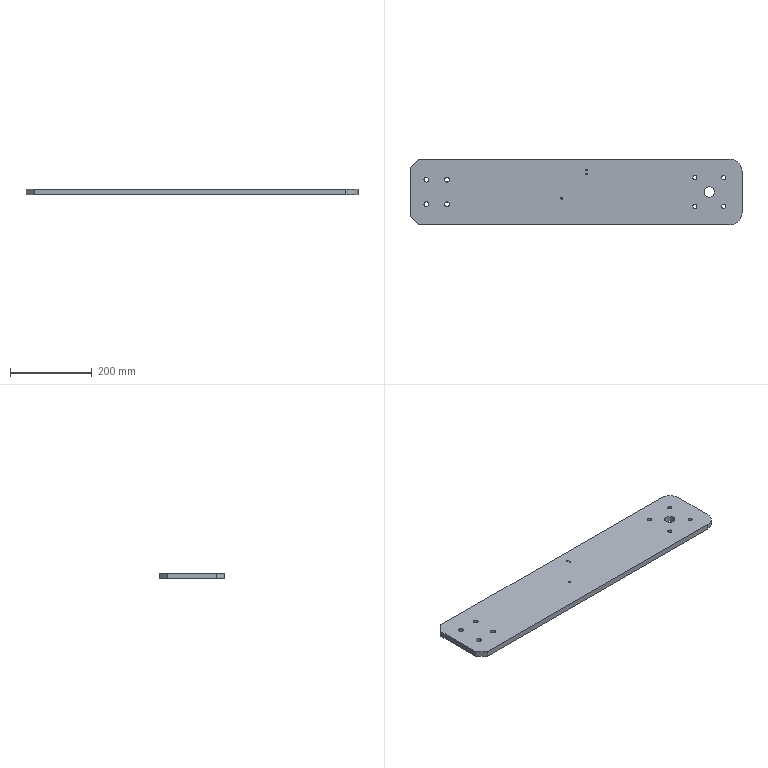Part | STEP file | Head plate 2 | 1 solid | 34 faces | box 810 x 160 x 14 mm | volume 1785161 mm3 | cylinder 26 | plane 8 | commonest cylinder face diameters 10 x8 12 x8 4 x4 5 x2 25 x2 60 x2
STEP:
#1=CARTESIAN_POINT('',(312.5,0.,14.));
#2=VERTEX_POINT('',#1);
#3=CARTESIAN_POINT('',(337.5,0.,14.));
#4=VERTEX_POINT('',#3);
#5=CARTESIAN_POINT('',(325.,0.,14.));
#6=DIRECTION('',(0.,0.,1.));
#7=DIRECTION('',(-1.,0.,0.));
#8=AXIS2_PLACEMENT_3D('',#5,#6,#7);
#9=CIRCLE('',#8,12.5);
#10=EDGE_CURVE('',#2,#4,#9,.T.);
#11=ORIENTED_EDGE('',*,*,#10,.T.);
#12=CARTESIAN_POINT('',(337.5,0.,0.));
#13=VERTEX_POINT('',#12);
#14=CARTESIAN_POINT('',(337.5,0.,14.));
#15=DIRECTION('',(0.,0.,-1.));
#16=VECTOR('',#15,1000.);
#17=LINE('',#14,#16);
#18=EDGE_CURVE('',#4,#13,#17,.T.);
#19=ORIENTED_EDGE('',*,*,#18,.T.);
#20=CARTESIAN_POINT('',(312.5,0.,0.));
#21=VERTEX_POINT('',#20);
#22=CARTESIAN_POINT('',(325.,0.,0.));
#23=DIRECTION('',(0.,0.,1.));
#24=DIRECTION('',(-1.,0.,0.));
#25=AXIS2_PLACEMENT_3D('',#22,#23,#24);
#26=CIRCLE('',#25,12.5);
#27=EDGE_CURVE('',#21,#13,#26,.T.);
#28=ORIENTED_EDGE('',*,*,#27,.F.);
#29=CARTESIAN_POINT('',(312.5,0.,14.));
#30=DIRECTION('',(0.,0.,-1.));
#31=VECTOR('',#30,1000.);
#32=LINE('',#29,#31);
#33=EDGE_CURVE('',#2,#21,#32,.T.);
#34=ORIENTED_EDGE('',*,*,#33,.F.);
#35=EDGE_LOOP('',(#11,#19,#28,#34));
#36=FACE_OUTER_BOUND('',#35,.T.);
#37=CARTESIAN_POINT('',(325.,0.,14.));
#38=DIRECTION('',(0.,0.,-1.));
#39=DIRECTION('',(-1.,0.,0.));
#40=AXIS2_PLACEMENT_3D('',#37,#38,#39);
#41=CYLINDRICAL_SURFACE('',#40,12.5);
#42=ADVANCED_FACE('',(#36),#41,.F.);
#43=CARTESIAN_POINT('',(355.,35.,14.));
#44=VERTEX_POINT('',#43);
#45=CARTESIAN_POINT('',(365.,35.,14.));
#46=VERTEX_POINT('',#45);
#47=CARTESIAN_POINT('',(360.,35.,14.));
#48=DIRECTION('',(0.,0.,1.));
#49=DIRECTION('',(-1.,0.,0.));
#50=AXIS2_PLACEMENT_3D('',#47,#48,#49);
#51=CIRCLE('',#50,5.);
#52=EDGE_CURVE('',#44,#46,#51,.T.);
#53=ORIENTED_EDGE('',*,*,#52,.T.);
#54=CARTESIAN_POINT('',(365.,35.,0.));
#55=VERTEX_POINT('',#54);
#56=CARTESIAN_POINT('',(365.,35.,14.));
#57=DIRECTION('',(0.,0.,-1.));
#58=VECTOR('',#57,1000.);
#59=LINE('',#56,#58);
#60=EDGE_CURVE('',#46,#55,#59,.T.);
#61=ORIENTED_EDGE('',*,*,#60,.T.);
#62=CARTESIAN_POINT('',(355.,35.,0.));
#63=VERTEX_POINT('',#62);
#64=CARTESIAN_POINT('',(360.,35.,0.));
#65=DIRECTION('',(0.,0.,1.));
#66=DIRECTION('',(-1.,0.,0.));
#67=AXIS2_PLACEMENT_3D('',#64,#65,#66);
#68=CIRCLE('',#67,5.);
#69=EDGE_CURVE('',#63,#55,#68,.T.);
#70=ORIENTED_EDGE('',*,*,#69,.F.);
#71=CARTESIAN_POINT('',(355.,35.,14.));
#72=DIRECTION('',(0.,0.,-1.));
#73=VECTOR('',#72,1000.);
#74=LINE('',#71,#73);
#75=EDGE_CURVE('',#44,#63,#74,.T.);
#76=ORIENTED_EDGE('',*,*,#75,.F.);
#77=EDGE_LOOP('',(#53,#61,#70,#76));
#78=FACE_OUTER_BOUND('',#77,.T.);
#79=CARTESIAN_POINT('',(360.,35.,14.));
#80=DIRECTION('',(0.,0.,-1.));
#81=DIRECTION('',(-1.,0.,0.));
#82=AXIS2_PLACEMENT_3D('',#79,#80,#81);
#83=CYLINDRICAL_SURFACE('',#82,5.);
#84=ADVANCED_FACE('',(#78),#83,.F.);
#85=CARTESIAN_POINT('',(285.,35.,14.));
#86=VERTEX_POINT('',#85);
#87=CARTESIAN_POINT('',(295.,35.,14.));
#88=VERTEX_POINT('',#87);
#89=CARTESIAN_POINT('',(290.,35.,14.));
#90=DIRECTION('',(0.,0.,1.));
#91=DIRECTION('',(-1.,0.,0.));
#92=AXIS2_PLACEMENT_3D('',#89,#90,#91);
#93=CIRCLE('',#92,5.);
#94=EDGE_CURVE('',#86,#88,#93,.T.);
#95=ORIENTED_EDGE('',*,*,#94,.T.);
#96=CARTESIAN_POINT('',(295.,35.,0.));
#97=VERTEX_POINT('',#96);
#98=CARTESIAN_POINT('',(295.,35.,14.));
#99=DIRECTION('',(0.,0.,-1.));
#100=VECTOR('',#99,1000.);
#101=LINE('',#98,#100);
#102=EDGE_CURVE('',#88,#97,#101,.T.);
#103=ORIENTED_EDGE('',*,*,#102,.T.);
#104=CARTESIAN_POINT('',(285.,35.,0.));
#105=VERTEX_POINT('',#104);
#106=CARTESIAN_POINT('',(290.,35.,0.));
#107=DIRECTION('',(0.,0.,1.));
#108=DIRECTION('',(-1.,0.,0.));
#109=AXIS2_PLACEMENT_3D('',#106,#107,#108);
#110=CIRCLE('',#109,5.);
#111=EDGE_CURVE('',#105,#97,#110,.T.);
#112=ORIENTED_EDGE('',*,*,#111,.F.);
#113=CARTESIAN_POINT('',(285.,35.,14.));
#114=DIRECTION('',(0.,0.,-1.));
#115=VECTOR('',#114,1000.);
#116=LINE('',#113,#115);
#117=EDGE_CURVE('',#86,#105,#116,.T.);
#118=ORIENTED_EDGE('',*,*,#117,.F.);
#119=EDGE_LOOP('',(#95,#103,#112,#118));
#120=FACE_OUTER_BOUND('',#119,.T.);
#121=CARTESIAN_POINT('',(290.,35.,14.));
#122=DIRECTION('',(0.,0.,-1.));
#123=DIRECTION('',(-1.,0.,0.));
#124=AXIS2_PLACEMENT_3D('',#121,#122,#123);
#125=CYLINDRICAL_SURFACE('',#124,5.);
#126=ADVANCED_FACE('',(#120),#125,.F.);
#127=CARTESIAN_POINT('',(285.,-35.,14.));
#128=VERTEX_POINT('',#127);
#129=CARTESIAN_POINT('',(295.,-35.,14.));
#130=VERTEX_POINT('',#129);
#131=CARTESIAN_POINT('',(290.,-35.,14.));
#132=DIRECTION('',(0.,0.,1.));
#133=DIRECTION('',(-1.,0.,0.));
#134=AXIS2_PLACEMENT_3D('',#131,#132,#133);
#135=CIRCLE('',#134,5.);
#136=EDGE_CURVE('',#128,#130,#135,.T.);
#137=ORIENTED_EDGE('',*,*,#136,.T.);
#138=CARTESIAN_POINT('',(295.,-35.,0.));
#139=VERTEX_POINT('',#138);
#140=CARTESIAN_POINT('',(295.,-35.,14.));
#141=DIRECTION('',(0.,0.,-1.));
#142=VECTOR('',#141,1000.);
#143=LINE('',#140,#142);
#144=EDGE_CURVE('',#130,#139,#143,.T.);
#145=ORIENTED_EDGE('',*,*,#144,.T.);
#146=CARTESIAN_POINT('',(285.,-35.,0.));
#147=VERTEX_POINT('',#146);
#148=CARTESIAN_POINT('',(290.,-35.,0.));
#149=DIRECTION('',(0.,0.,1.));
#150=DIRECTION('',(-1.,0.,0.));
#151=AXIS2_PLACEMENT_3D('',#148,#149,#150);
#152=CIRCLE('',#151,5.);
#153=EDGE_CURVE('',#147,#139,#152,.T.);
#154=ORIENTED_EDGE('',*,*,#153,.F.);
#155=CARTESIAN_POINT('',(285.,-35.,14.));
#156=DIRECTION('',(0.,0.,-1.));
#157=VECTOR('',#156,1000.);
#158=LINE('',#155,#157);
#159=EDGE_CURVE('',#128,#147,#158,.T.);
#160=ORIENTED_EDGE('',*,*,#159,.F.);
#161=EDGE_LOOP('',(#137,#145,#154,#160));
#162=FACE_OUTER_BOUND('',#161,.T.);
#163=CARTESIAN_POINT('',(290.,-35.,14.));
#164=DIRECTION('',(0.,0.,-1.));
#165=DIRECTION('',(-1.,0.,0.));
#166=AXIS2_PLACEMENT_3D('',#163,#164,#165);
#167=CYLINDRICAL_SURFACE('',#166,5.);
#168=ADVANCED_FACE('',(#162),#167,.F.);
#169=CARTESIAN_POINT('',(355.,-35.,14.));
#170=VERTEX_POINT('',#169);
#171=CARTESIAN_POINT('',(365.,-35.,14.));
#172=VERTEX_POINT('',#171);
#173=CARTESIAN_POINT('',(360.,-35.,14.));
#174=DIRECTION('',(0.,0.,1.));
#175=DIRECTION('',(-1.,0.,0.));
#176=AXIS2_PLACEMENT_3D('',#173,#174,#175);
#177=CIRCLE('',#176,5.);
#178=EDGE_CURVE('',#170,#172,#177,.T.);
#179=ORIENTED_EDGE('',*,*,#178,.T.);
#180=CARTESIAN_POINT('',(365.,-35.,0.));
#181=VERTEX_POINT('',#180);
#182=CARTESIAN_POINT('',(365.,-35.,14.));
#183=DIRECTION('',(0.,0.,-1.));
#184=VECTOR('',#183,1000.);
#185=LINE('',#182,#184);
#186=EDGE_CURVE('',#172,#181,#185,.T.);
#187=ORIENTED_EDGE('',*,*,#186,.T.);
#188=CARTESIAN_POINT('',(355.,-35.,0.));
#189=VERTEX_POINT('',#188);
#190=CARTESIAN_POINT('',(360.,-35.,0.));
#191=DIRECTION('',(0.,0.,1.));
#192=DIRECTION('',(-1.,0.,0.));
#193=AXIS2_PLACEMENT_3D('',#190,#191,#192);
#194=CIRCLE('',#193,5.);
#195=EDGE_CURVE('',#189,#181,#194,.T.);
#196=ORIENTED_EDGE('',*,*,#195,.F.);
#197=CARTESIAN_POINT('',(355.,-35.,14.));
#198=DIRECTION('',(0.,0.,-1.));
#199=VECTOR('',#198,1000.);
#200=LINE('',#197,#199);
#201=EDGE_CURVE('',#170,#189,#200,.T.);
#202=ORIENTED_EDGE('',*,*,#201,.F.);
#203=EDGE_LOOP('',(#179,#187,#196,#202));
#204=FACE_OUTER_BOUND('',#203,.T.);
#205=CARTESIAN_POINT('',(360.,-35.,14.));
#206=DIRECTION('',(0.,0.,-1.));
#207=DIRECTION('',(-1.,0.,0.));
#208=AXIS2_PLACEMENT_3D('',#205,#206,#207);
#209=CYLINDRICAL_SURFACE('',#208,5.);
#210=ADVANCED_FACE('',(#204),#209,.F.);
#211=CARTESIAN_POINT('',(-37.5,-15.,0.));
#212=VERTEX_POINT('',#211);
#213=CARTESIAN_POINT('',(-32.5,-15.,0.));
#214=VERTEX_POINT('',#213);
#215=CARTESIAN_POINT('',(-35.,-15.,0.));
#216=DIRECTION('',(0.,0.,1.));
#217=DIRECTION('',(1.,0.,0.));
#218=AXIS2_PLACEMENT_3D('',#215,#216,#217);
#219=CIRCLE('',#218,2.5);
#220=EDGE_CURVE('',#212,#214,#219,.T.);
#221=ORIENTED_EDGE('',*,*,#220,.F.);
#222=CARTESIAN_POINT('',(-37.5,-15.,14.));
#223=VERTEX_POINT('',#222);
#224=CARTESIAN_POINT('',(-37.5,-15.,-1.));
#225=DIRECTION('',(0.,0.,1.));
#226=VECTOR('',#225,1000.);
#227=LINE('',#224,#226);
#228=EDGE_CURVE('',#212,#223,#227,.T.);
#229=ORIENTED_EDGE('',*,*,#228,.T.);
#230=CARTESIAN_POINT('',(-32.5,-15.,14.));
#231=VERTEX_POINT('',#230);
#232=CARTESIAN_POINT('',(-35.,-15.,14.));
#233=DIRECTION('',(0.,0.,1.));
#234=DIRECTION('',(1.,0.,0.));
#235=AXIS2_PLACEMENT_3D('',#232,#233,#234);
#236=CIRCLE('',#235,2.5);
#237=EDGE_CURVE('',#223,#231,#236,.T.);
#238=ORIENTED_EDGE('',*,*,#237,.T.);
#239=CARTESIAN_POINT('',(-32.5,-15.,-1.));
#240=DIRECTION('',(0.,0.,1.));
#241=VECTOR('',#240,1000.);
#242=LINE('',#239,#241);
#243=EDGE_CURVE('',#214,#231,#242,.T.);
#244=ORIENTED_EDGE('',*,*,#243,.F.);
#245=EDGE_LOOP('',(#221,#229,#238,#244));
#246=FACE_OUTER_BOUND('',#245,.T.);
#247=CARTESIAN_POINT('',(-35.,-15.,-1.));
#248=DIRECTION('',(0.,0.,1.));
#249=DIRECTION('',(1.,0.,0.));
#250=AXIS2_PLACEMENT_3D('',#247,#248,#249);
#251=CYLINDRICAL_SURFACE('',#250,2.5);
#252=ADVANCED_FACE('',(#246),#251,.F.);
#253=CARTESIAN_POINT('',(-371.,30.,0.));
#254=VERTEX_POINT('',#253);
#255=CARTESIAN_POINT('',(-359.,30.,0.));
#256=VERTEX_POINT('',#255);
#257=CARTESIAN_POINT('',(-365.,30.,0.));
#258=DIRECTION('',(0.,0.,1.));
#259=DIRECTION('',(1.,0.,0.));
#260=AXIS2_PLACEMENT_3D('',#257,#258,#259);
#261=CIRCLE('',#260,6.);
#262=EDGE_CURVE('',#254,#256,#261,.T.);
#263=ORIENTED_EDGE('',*,*,#262,.F.);
#264=CARTESIAN_POINT('',(-371.,30.,14.));
#265=VERTEX_POINT('',#264);
#266=CARTESIAN_POINT('',(-371.,30.,-1.));
#267=DIRECTION('',(0.,0.,1.));
#268=VECTOR('',#267,1000.);
#269=LINE('',#266,#268);
#270=EDGE_CURVE('',#254,#265,#269,.T.);
#271=ORIENTED_EDGE('',*,*,#270,.T.);
#272=CARTESIAN_POINT('',(-359.,30.,14.));
#273=VERTEX_POINT('',#272);
#274=CARTESIAN_POINT('',(-365.,30.,14.));
#275=DIRECTION('',(0.,0.,1.));
#276=DIRECTION('',(1.,0.,0.));
#277=AXIS2_PLACEMENT_3D('',#274,#275,#276);
#278=CIRCLE('',#277,6.);
#279=EDGE_CURVE('',#265,#273,#278,.T.);
#280=ORIENTED_EDGE('',*,*,#279,.T.);
#281=CARTESIAN_POINT('',(-359.,30.,-1.));
#282=DIRECTION('',(0.,0.,1.));
#283=VECTOR('',#282,1000.);
#284=LINE('',#281,#283);
#285=EDGE_CURVE('',#256,#273,#284,.T.);
#286=ORIENTED_EDGE('',*,*,#285,.F.);
#287=EDGE_LOOP('',(#263,#271,#280,#286));
#288=FACE_OUTER_BOUND('',#287,.T.);
#289=CARTESIAN_POINT('',(-365.,30.,-1.));
#290=DIRECTION('',(0.,0.,1.));
#291=DIRECTION('',(1.,0.,0.));
#292=AXIS2_PLACEMENT_3D('',#289,#290,#291);
#293=CYLINDRICAL_SURFACE('',#292,6.);
#294=ADVANCED_FACE('',(#288),#293,.F.);
#295=CARTESIAN_POINT('',(-321.,30.,0.));
#296=VERTEX_POINT('',#295);
#297=CARTESIAN_POINT('',(-309.,30.,0.));
#298=VERTEX_POINT('',#297);
#299=CARTESIAN_POINT('',(-315.,30.,0.));
#300=DIRECTION('',(0.,0.,1.));
#301=DIRECTION('',(1.,0.,0.));
#302=AXIS2_PLACEMENT_3D('',#299,#300,#301);
#303=CIRCLE('',#302,6.);
#304=EDGE_CURVE('',#296,#298,#303,.T.);
#305=ORIENTED_EDGE('',*,*,#304,.F.);
#306=CARTESIAN_POINT('',(-321.,30.,14.));
#307=VERTEX_POINT('',#306);
#308=CARTESIAN_POINT('',(-321.,30.,-1.));
#309=DIRECTION('',(0.,0.,1.));
#310=VECTOR('',#309,1000.);
#311=LINE('',#308,#310);
#312=EDGE_CURVE('',#296,#307,#311,.T.);
#313=ORIENTED_EDGE('',*,*,#312,.T.);
#314=CARTESIAN_POINT('',(-309.,30.,14.));
#315=VERTEX_POINT('',#314);
#316=CARTESIAN_POINT('',(-315.,30.,14.));
#317=DIRECTION('',(0.,0.,1.));
#318=DIRECTION('',(1.,0.,0.));
#319=AXIS2_PLACEMENT_3D('',#316,#317,#318);
#320=CIRCLE('',#319,6.);
#321=EDGE_CURVE('',#307,#315,#320,.T.);
#322=ORIENTED_EDGE('',*,*,#321,.T.);
#323=CARTESIAN_POINT('',(-309.,30.,-1.));
#324=DIRECTION('',(0.,0.,1.));
#325=VECTOR('',#324,1000.);
#326=LINE('',#323,#325);
#327=EDGE_CURVE('',#298,#315,#326,.T.);
#328=ORIENTED_EDGE('',*,*,#327,.F.);
#329=EDGE_LOOP('',(#305,#313,#322,#328));
#330=FACE_OUTER_BOUND('',#329,.T.);
#331=CARTESIAN_POINT('',(-315.,30.,-1.));
#332=DIRECTION('',(0.,0.,1.));
#333=DIRECTION('',(1.,0.,0.));
#334=AXIS2_PLACEMENT_3D('',#331,#332,#333);
#335=CYLINDRICAL_SURFACE('',#334,6.);
#336=ADVANCED_FACE('',(#330),#335,.F.);
#337=CARTESIAN_POINT('',(-371.,-30.,0.));
#338=VERTEX_POINT('',#337);
#339=CARTESIAN_POINT('',(-359.,-30.,0.));
#340=VERTEX_POINT('',#339);
#341=CARTESIAN_POINT('',(-365.,-30.,0.));
#342=DIRECTION('',(0.,0.,1.));
#343=DIRECTION('',(1.,0.,0.));
#344=AXIS2_PLACEMENT_3D('',#341,#342,#343);
#345=CIRCLE('',#344,6.);
#346=EDGE_CURVE('',#338,#340,#345,.T.);
#347=ORIENTED_EDGE('',*,*,#346,.F.);
#348=CARTESIAN_POINT('',(-371.,-30.,14.));
#349=VERTEX_POINT('',#348);
#350=CARTESIAN_POINT('',(-371.,-30.,-1.));
#351=DIRECTION('',(0.,0.,1.));
#352=VECTOR('',#351,1000.);
#353=LINE('',#350,#352);
#354=EDGE_CURVE('',#338,#349,#353,.T.);
#355=ORIENTED_EDGE('',*,*,#354,.T.);
#356=CARTESIAN_POINT('',(-359.,-30.,14.));
#357=VERTEX_POINT('',#356);
#358=CARTESIAN_POINT('',(-365.,-30.,14.));
#359=DIRECTION('',(0.,0.,1.));
#360=DIRECTION('',(1.,0.,0.));
#361=AXIS2_PLACEMENT_3D('',#358,#359,#360);
#362=CIRCLE('',#361,6.);
#363=EDGE_CURVE('',#349,#357,#362,.T.);
#364=ORIENTED_EDGE('',*,*,#363,.T.);
#365=CARTESIAN_POINT('',(-359.,-30.,-1.));
#366=DIRECTION('',(0.,0.,1.));
#367=VECTOR('',#366,1000.);
#368=LINE('',#365,#367);
#369=EDGE_CURVE('',#340,#357,#368,.T.);
#370=ORIENTED_EDGE('',*,*,#369,.F.);
#371=EDGE_LOOP('',(#347,#355,#364,#370));
#372=FACE_OUTER_BOUND('',#371,.T.);
#373=CARTESIAN_POINT('',(-365.,-30.,-1.));
#374=DIRECTION('',(0.,0.,1.));
#375=DIRECTION('',(1.,0.,0.));
#376=AXIS2_PLACEMENT_3D('',#373,#374,#375);
#377=CYLINDRICAL_SURFACE('',#376,6.);
#378=ADVANCED_FACE('',(#372),#377,.F.);
#379=CARTESIAN_POINT('',(-321.,-30.,0.));
#380=VERTEX_POINT('',#379);
#381=CARTESIAN_POINT('',(-309.,-30.,0.));
#382=VERTEX_POINT('',#381);
#383=CARTESIAN_POINT('',(-315.,-30.,0.));
#384=DIRECTION('',(0.,0.,1.));
#385=DIRECTION('',(1.,0.,0.));
#386=AXIS2_PLACEMENT_3D('',#383,#384,#385);
#387=CIRCLE('',#386,6.);
#388=EDGE_CURVE('',#380,#382,#387,.T.);
#389=ORIENTED_EDGE('',*,*,#388,.F.);
#390=CARTESIAN_POINT('',(-321.,-30.,14.));
#391=VERTEX_POINT('',#390);
#392=CARTESIAN_POINT('',(-321.,-30.,-1.));
#393=DIRECTION('',(0.,0.,1.));
#394=VECTOR('',#393,1000.);
#395=LINE('',#392,#394);
#396=EDGE_CURVE('',#380,#391,#395,.T.);
#397=ORIENTED_EDGE('',*,*,#396,.T.);
#398=CARTESIAN_POINT('',(-309.,-30.,14.));
#399=VERTEX_POINT('',#398);
#400=CARTESIAN_POINT('',(-315.,-30.,14.));
#401=DIRECTION('',(0.,0.,1.));
#402=DIRECTION('',(1.,0.,0.));
#403=AXIS2_PLACEMENT_3D('',#400,#401,#402);
#404=CIRCLE('',#403,6.);
#405=EDGE_CURVE('',#391,#399,#404,.T.);
#406=ORIENTED_EDGE('',*,*,#405,.T.);
#407=CARTESIAN_POINT('',(-309.,-30.,-1.));
#408=DIRECTION('',(0.,0.,1.));
#409=VECTOR('',#408,1000.);
#410=LINE('',#407,#409);
#411=EDGE_CURVE('',#382,#399,#410,.T.);
#412=ORIENTED_EDGE('',*,*,#411,.F.);
#413=EDGE_LOOP('',(#389,#397,#406,#412));
#414=FACE_OUTER_BOUND('',#413,.T.);
#415=CARTESIAN_POINT('',(-315.,-30.,-1.));
#416=DIRECTION('',(0.,0.,1.));
#417=DIRECTION('',(1.,0.,0.));
#418=AXIS2_PLACEMENT_3D('',#415,#416,#417);
#419=CYLINDRICAL_SURFACE('',#418,6.);
#420=ADVANCED_FACE('',(#414),#419,.F.);
#421=CARTESIAN_POINT('',(23.,54.,14.));
#422=VERTEX_POINT('',#421);
#423=CARTESIAN_POINT('',(27.,54.,14.));
#424=VERTEX_POINT('',#423);
#425=CARTESIAN_POINT('',(25.,54.,14.));
#426=DIRECTION('',(0.,0.,1.));
#427=DIRECTION('',(-1.,0.,0.));
#428=AXIS2_PLACEMENT_3D('',#425,#426,#427);
#429=CIRCLE('',#428,2.);
#430=EDGE_CURVE('',#422,#424,#429,.T.);
#431=ORIENTED_EDGE('',*,*,#430,.T.);
#432=CARTESIAN_POINT('',(27.,54.,0.));
#433=VERTEX_POINT('',#432);
#434=CARTESIAN_POINT('',(27.,54.,20.));
#435=DIRECTION('',(0.,0.,-1.));
#436=VECTOR('',#435,1000.);
#437=LINE('',#434,#436);
#438=EDGE_CURVE('',#424,#433,#437,.T.);
#439=ORIENTED_EDGE('',*,*,#438,.T.);
#440=CARTESIAN_POINT('',(23.,54.,0.));
#441=VERTEX_POINT('',#440);
#442=CARTESIAN_POINT('',(25.,54.,0.));
#443=DIRECTION('',(0.,0.,1.));
#444=DIRECTION('',(-1.,0.,0.));
#445=AXIS2_PLACEMENT_3D('',#442,#443,#444);
#446=CIRCLE('',#445,2.);
#447=EDGE_CURVE('',#441,#433,#446,.T.);
#448=ORIENTED_EDGE('',*,*,#447,.F.);
#449=CARTESIAN_POINT('',(23.,54.,20.));
#450=DIRECTION('',(0.,0.,-1.));
#451=VECTOR('',#450,1000.);
#452=LINE('',#449,#451);
#453=EDGE_CURVE('',#422,#441,#452,.T.);
#454=ORIENTED_EDGE('',*,*,#453,.F.);
#455=EDGE_LOOP('',(#431,#439,#448,#454));
#456=FACE_OUTER_BOUND('',#455,.T.);
#457=CARTESIAN_POINT('',(25.,54.,20.));
#458=DIRECTION('',(0.,0.,-1.));
#459=DIRECTION('',(-1.,0.,0.));
#460=AXIS2_PLACEMENT_3D('',#457,#458,#459);
#461=CYLINDRICAL_SURFACE('',#460,2.);
#462=ADVANCED_FACE('',(#456),#461,.F.);
#463=CARTESIAN_POINT('',(23.,44.,14.));
#464=VERTEX_POINT('',#463);
#465=CARTESIAN_POINT('',(27.,44.,14.));
#466=VERTEX_POINT('',#465);
#467=CARTESIAN_POINT('',(25.,44.,14.));
#468=DIRECTION('',(0.,0.,1.));
#469=DIRECTION('',(-1.,0.,0.));
#470=AXIS2_PLACEMENT_3D('',#467,#468,#469);
#471=CIRCLE('',#470,2.);
#472=EDGE_CURVE('',#464,#466,#471,.T.);
#473=ORIENTED_EDGE('',*,*,#472,.T.);
#474=CARTESIAN_POINT('',(27.,44.,0.));
#475=VERTEX_POINT('',#474);
#476=CARTESIAN_POINT('',(27.,44.,20.));
#477=DIRECTION('',(0.,0.,-1.));
#478=VECTOR('',#477,1000.);
#479=LINE('',#476,#478);
#480=EDGE_CURVE('',#466,#475,#479,.T.);
#481=ORIENTED_EDGE('',*,*,#480,.T.);
#482=CARTESIAN_POINT('',(23.,44.,0.));
#483=VERTEX_POINT('',#482);
#484=CARTESIAN_POINT('',(25.,44.,0.));
#485=DIRECTION('',(0.,0.,1.));
#486=DIRECTION('',(-1.,0.,0.));
#487=AXIS2_PLACEMENT_3D('',#484,#485,#486);
#488=CIRCLE('',#487,2.);
#489=EDGE_CURVE('',#483,#475,#488,.T.);
#490=ORIENTED_EDGE('',*,*,#489,.F.);
#491=CARTESIAN_POINT('',(23.,44.,20.));
#492=DIRECTION('',(0.,0.,-1.));
#493=VECTOR('',#492,1000.);
#494=LINE('',#491,#493);
#495=EDGE_CURVE('',#464,#483,#494,.T.);
#496=ORIENTED_EDGE('',*,*,#495,.F.);
#497=EDGE_LOOP('',(#473,#481,#490,#496));
#498=FACE_OUTER_BOUND('',#497,.T.);
#499=CARTESIAN_POINT('',(25.,44.,20.));
#500=DIRECTION('',(0.,0.,-1.));
#501=DIRECTION('',(-1.,0.,0.));
#502=AXIS2_PLACEMENT_3D('',#499,#500,#501);
#503=CYLINDRICAL_SURFACE('',#502,2.);
#504=ADVANCED_FACE('',(#498),#503,.F.);
#505=CARTESIAN_POINT('',(-385.,-80.,14.));
#506=VERTEX_POINT('',#505);
#507=CARTESIAN_POINT('',(-405.,-60.,14.));
#508=VERTEX_POINT('',#507);
#509=CARTESIAN_POINT('',(-385.,-80.,14.));
#510=DIRECTION('',(-0.7071,0.7071,0.));
#511=VECTOR('',#510,1000.);
#512=LINE('',#509,#511);
#513=EDGE_CURVE('',#506,#508,#512,.T.);
#514=ORIENTED_EDGE('',*,*,#513,.F.);
#515=CARTESIAN_POINT('',(375.,-80.,14.));
#516=VERTEX_POINT('',#515);
#517=CARTESIAN_POINT('',(405.,-80.,14.));
#518=DIRECTION('',(-1.,0.,0.));
#519=VECTOR('',#518,1000.);
#520=LINE('',#517,#519);
#521=EDGE_CURVE('',#516,#506,#520,.T.);
#522=ORIENTED_EDGE('',*,*,#521,.F.);
#523=CARTESIAN_POINT('',(405.,-50.,14.));
#524=VERTEX_POINT('',#523);
#525=CARTESIAN_POINT('',(375.,-50.,14.));
#526=DIRECTION('',(0.,0.,-1.));
#527=DIRECTION('',(-1.,0.,0.));
#528=AXIS2_PLACEMENT_3D('',#525,#526,#527);
#529=CIRCLE('',#528,30.);
#530=EDGE_CURVE('',#524,#516,#529,.T.);
#531=ORIENTED_EDGE('',*,*,#530,.F.);
#532=CARTESIAN_POINT('',(405.,50.,14.));
#533=VERTEX_POINT('',#532);
#534=CARTESIAN_POINT('',(405.,-80.,14.));
#535=DIRECTION('',(0.,-1.,0.));
#536=VECTOR('',#535,1000.);
#537=LINE('',#534,#536);
#538=EDGE_CURVE('',#533,#524,#537,.T.);
#539=ORIENTED_EDGE('',*,*,#538,.F.);
#540=CARTESIAN_POINT('',(375.,80.,14.));
#541=VERTEX_POINT('',#540);
#542=CARTESIAN_POINT('',(375.,50.,14.));
#543=DIRECTION('',(0.,0.,-1.));
#544=DIRECTION('',(-1.,0.,0.));
#545=AXIS2_PLACEMENT_3D('',#542,#543,#544);
#546=CIRCLE('',#545,30.);
#547=EDGE_CURVE('',#541,#533,#546,.T.);
#548=ORIENTED_EDGE('',*,*,#547,.F.);
#549=CARTESIAN_POINT('',(-385.,80.,14.));
#550=VERTEX_POINT('',#549);
#551=CARTESIAN_POINT('',(405.,80.,14.));
#552=DIRECTION('',(1.,0.,0.));
#553=VECTOR('',#552,1000.);
#554=LINE('',#551,#553);
#555=EDGE_CURVE('',#550,#541,#554,.T.);
#556=ORIENTED_EDGE('',*,*,#555,.F.);
#557=CARTESIAN_POINT('',(-405.,60.,14.));
#558=VERTEX_POINT('',#557);
#559=CARTESIAN_POINT('',(-405.,60.,14.));
#560=DIRECTION('',(0.7071,0.7071,0.));
#561=VECTOR('',#560,1000.);
#562=LINE('',#559,#561);
#563=EDGE_CURVE('',#558,#550,#562,.T.);
#564=ORIENTED_EDGE('',*,*,#563,.F.);
#565=CARTESIAN_POINT('',(-405.,-80.,14.));
#566=DIRECTION('',(0.,1.,0.));
#567=VECTOR('',#566,1000.);
#568=LINE('',#565,#567);
#569=EDGE_CURVE('',#508,#558,#568,.T.);
#570=ORIENTED_EDGE('',*,*,#569,.F.);
#571=EDGE_LOOP('',(#514,#522,#531,#539,#548,#556,#564,#570));
#572=FACE_OUTER_BOUND('',#571,.T.);
#573=ORIENTED_EDGE('',*,*,#10,.F.);
#574=CARTESIAN_POINT('',(325.,0.,14.));
#575=DIRECTION('',(0.,0.,1.));
#576=DIRECTION('',(-1.,0.,0.));
#577=AXIS2_PLACEMENT_3D('',#574,#575,#576);
#578=CIRCLE('',#577,12.5);
#579=EDGE_CURVE('',#4,#2,#578,.T.);
#580=ORIENTED_EDGE('',*,*,#579,.F.);
#581=EDGE_LOOP('',(#573,#580));
#582=FACE_BOUND('',#581,.T.);
#583=ORIENTED_EDGE('',*,*,#52,.F.);
#584=CARTESIAN_POINT('',(360.,35.,14.));
#585=DIRECTION('',(0.,0.,1.));
#586=DIRECTION('',(-1.,0.,0.));
#587=AXIS2_PLACEMENT_3D('',#584,#585,#586);
#588=CIRCLE('',#587,5.);
#589=EDGE_CURVE('',#46,#44,#588,.T.);
#590=ORIENTED_EDGE('',*,*,#589,.F.);
#591=EDGE_LOOP('',(#583,#590));
#592=FACE_BOUND('',#591,.T.);
#593=ORIENTED_EDGE('',*,*,#94,.F.);
#594=CARTESIAN_POINT('',(290.,35.,14.));
#595=DIRECTION('',(0.,0.,1.));
#596=DIRECTION('',(-1.,0.,0.));
#597=AXIS2_PLACEMENT_3D('',#594,#595,#596);
#598=CIRCLE('',#597,5.);
#599=EDGE_CURVE('',#88,#86,#598,.T.);
#600=ORIENTED_EDGE('',*,*,#599,.F.);
#601=EDGE_LOOP('',(#593,#600));
#602=FACE_BOUND('',#601,.T.);
#603=ORIENTED_EDGE('',*,*,#136,.F.);
#604=CARTESIAN_POINT('',(290.,-35.,14.));
#605=DIRECTION('',(0.,0.,1.));
#606=DIRECTION('',(-1.,0.,0.));
#607=AXIS2_PLACEMENT_3D('',#604,#605,#606);
#608=CIRCLE('',#607,5.);
#609=EDGE_CURVE('',#130,#128,#608,.T.);
#610=ORIENTED_EDGE('',*,*,#609,.F.);
#611=EDGE_LOOP('',(#603,#610));
#612=FACE_BOUND('',#611,.T.);
#613=ORIENTED_EDGE('',*,*,#178,.F.);
#614=CARTESIAN_POINT('',(360.,-35.,14.));
#615=DIRECTION('',(0.,0.,1.));
#616=DIRECTION('',(-1.,0.,0.));
#617=AXIS2_PLACEMENT_3D('',#614,#615,#616);
#618=CIRCLE('',#617,5.);
#619=EDGE_CURVE('',#172,#170,#618,.T.);
#620=ORIENTED_EDGE('',*,*,#619,.F.);
#621=EDGE_LOOP('',(#613,#620));
#622=FACE_BOUND('',#621,.T.);
#623=CARTESIAN_POINT('',(-35.,-15.,14.));
#624=DIRECTION('',(0.,0.,1.));
#625=DIRECTION('',(1.,0.,0.));
#626=AXIS2_PLACEMENT_3D('',#623,#624,#625);
#627=CIRCLE('',#626,2.5);
#628=EDGE_CURVE('',#231,#223,#627,.T.);
#629=ORIENTED_EDGE('',*,*,#628,.F.);
#630=ORIENTED_EDGE('',*,*,#237,.F.);
#631=EDGE_LOOP('',(#629,#630));
#632=FACE_BOUND('',#631,.T.);
#633=CARTESIAN_POINT('',(-365.,30.,14.));
#634=DIRECTION('',(0.,0.,1.));
#635=DIRECTION('',(1.,0.,0.));
#636=AXIS2_PLACEMENT_3D('',#633,#634,#635);
#637=CIRCLE('',#636,6.);
#638=EDGE_CURVE('',#273,#265,#637,.T.);
#639=ORIENTED_EDGE('',*,*,#638,.F.);
#640=ORIENTED_EDGE('',*,*,#279,.F.);
#641=EDGE_LOOP('',(#639,#640));
#642=FACE_BOUND('',#641,.T.);
#643=CARTESIAN_POINT('',(-315.,30.,14.));
#644=DIRECTION('',(0.,0.,1.));
#645=DIRECTION('',(1.,0.,0.));
#646=AXIS2_PLACEMENT_3D('',#643,#644,#645);
#647=CIRCLE('',#646,6.);
#648=EDGE_CURVE('',#315,#307,#647,.T.);
#649=ORIENTED_EDGE('',*,*,#648,.F.);
#650=ORIENTED_EDGE('',*,*,#321,.F.);
#651=EDGE_LOOP('',(#649,#650));
#652=FACE_BOUND('',#651,.T.);
#653=CARTESIAN_POINT('',(-365.,-30.,14.));
#654=DIRECTION('',(0.,0.,1.));
#655=DIRECTION('',(1.,0.,0.));
#656=AXIS2_PLACEMENT_3D('',#653,#654,#655);
#657=CIRCLE('',#656,6.);
#658=EDGE_CURVE('',#357,#349,#657,.T.);
#659=ORIENTED_EDGE('',*,*,#658,.F.);
#660=ORIENTED_EDGE('',*,*,#363,.F.);
#661=EDGE_LOOP('',(#659,#660));
#662=FACE_BOUND('',#661,.T.);
#663=CARTESIAN_POINT('',(-315.,-30.,14.));
#664=DIRECTION('',(0.,0.,1.));
#665=DIRECTION('',(1.,0.,0.));
#666=AXIS2_PLACEMENT_3D('',#663,#664,#665);
#667=CIRCLE('',#666,6.);
#668=EDGE_CURVE('',#399,#391,#667,.T.);
#669=ORIENTED_EDGE('',*,*,#668,.F.);
#670=ORIENTED_EDGE('',*,*,#405,.F.);
#671=EDGE_LOOP('',(#669,#670));
#672=FACE_BOUND('',#671,.T.);
#673=ORIENTED_EDGE('',*,*,#430,.F.);
#674=CARTESIAN_POINT('',(25.,54.,14.));
#675=DIRECTION('',(0.,0.,1.));
#676=DIRECTION('',(-1.,0.,0.));
#677=AXIS2_PLACEMENT_3D('',#674,#675,#676);
#678=CIRCLE('',#677,2.);
#679=EDGE_CURVE('',#424,#422,#678,.T.);
#680=ORIENTED_EDGE('',*,*,#679,.F.);
#681=EDGE_LOOP('',(#673,#680));
#682=FACE_BOUND('',#681,.T.);
#683=ORIENTED_EDGE('',*,*,#472,.F.);
#684=CARTESIAN_POINT('',(25.,44.,14.));
#685=DIRECTION('',(0.,0.,1.));
#686=DIRECTION('',(-1.,0.,0.));
#687=AXIS2_PLACEMENT_3D('',#684,#685,#686);
#688=CIRCLE('',#687,2.);
#689=EDGE_CURVE('',#466,#464,#688,.T.);
#690=ORIENTED_EDGE('',*,*,#689,.F.);
#691=EDGE_LOOP('',(#683,#690));
#692=FACE_BOUND('',#691,.T.);
#693=CARTESIAN_POINT('',(405.,-80.,14.));
#694=DIRECTION('',(0.,0.,-1.));
#695=DIRECTION('',(-1.,0.,0.));
#696=AXIS2_PLACEMENT_3D('',#693,#694,#695);
#697=PLANE('',#696);
#698=ADVANCED_FACE('',(#572,#582,#592,#602,#612,#622,#632,#642,#652,#662,#672,#682,#692),#697,.F.);
#699=CARTESIAN_POINT('',(-405.,-60.,0.));
#700=VERTEX_POINT('',#699);
#701=CARTESIAN_POINT('',(-405.,-60.,14.));
#702=DIRECTION('',(0.,0.,-1.));
#703=VECTOR('',#702,1000.);
#704=LINE('',#701,#703);
#705=EDGE_CURVE('',#508,#700,#704,.T.);
#706=ORIENTED_EDGE('',*,*,#705,.F.);
#707=ORIENTED_EDGE('',*,*,#569,.T.);
#708=CARTESIAN_POINT('',(-405.,60.,0.));
#709=VERTEX_POINT('',#708);
#710=CARTESIAN_POINT('',(-405.,60.,14.));
#711=DIRECTION('',(0.,0.,1.));
#712=VECTOR('',#711,1000.);
#713=LINE('',#710,#712);
#714=EDGE_CURVE('',#709,#558,#713,.T.);
#715=ORIENTED_EDGE('',*,*,#714,.F.);
#716=CARTESIAN_POINT('',(-405.,80.,0.));
#717=DIRECTION('',(0.,1.,0.));
#718=VECTOR('',#717,1000.);
#719=LINE('',#716,#718);
#720=EDGE_CURVE('',#700,#709,#719,.T.);
#721=ORIENTED_EDGE('',*,*,#720,.F.);
#722=EDGE_LOOP('',(#706,#707,#715,#721));
#723=FACE_OUTER_BOUND('',#722,.T.);
#724=CARTESIAN_POINT('',(-405.,80.,14.));
#725=DIRECTION('',(1.,0.,0.));
#726=DIRECTION('',(0.,0.,-1.));
#727=AXIS2_PLACEMENT_3D('',#724,#725,#726);
#728=PLANE('',#727);
#729=ADVANCED_FACE('',(#723),#728,.F.);
#730=ORIENTED_EDGE('',*,*,#705,.T.);
#731=CARTESIAN_POINT('',(-385.,-80.,0.));
#732=VERTEX_POINT('',#731);
#733=CARTESIAN_POINT('',(-385.,-80.,0.));
#734=DIRECTION('',(-0.7071,0.7071,0.));
#735=VECTOR('',#734,1000.);
#736=LINE('',#733,#735);
#737=EDGE_CURVE('',#732,#700,#736,.T.);
#738=ORIENTED_EDGE('',*,*,#737,.F.);
#739=CARTESIAN_POINT('',(-385.,-80.,14.));
#740=DIRECTION('',(0.,0.,-1.));
#741=VECTOR('',#740,1000.);
#742=LINE('',#739,#741);
#743=EDGE_CURVE('',#506,#732,#742,.T.);
#744=ORIENTED_EDGE('',*,*,#743,.F.);
#745=ORIENTED_EDGE('',*,*,#513,.T.);
#746=EDGE_LOOP('',(#730,#738,#744,#745));
#747=FACE_OUTER_BOUND('',#746,.T.);
#748=CARTESIAN_POINT('',(-385.,-80.,14.));
#749=DIRECTION('',(0.7071,0.7071,0.));
#750=DIRECTION('',(-0.7071,0.7071,0.));
#751=AXIS2_PLACEMENT_3D('',#748,#749,#750);
#752=PLANE('',#751);
#753=ADVANCED_FACE('',(#747),#752,.F.);
#754=ORIENTED_EDGE('',*,*,#743,.T.);
#755=CARTESIAN_POINT('',(375.,-80.,0.));
#756=VERTEX_POINT('',#755);
#757=CARTESIAN_POINT('',(405.,-80.,0.));
#758=DIRECTION('',(-1.,0.,0.));
#759=VECTOR('',#758,1000.);
#760=LINE('',#757,#759);
#761=EDGE_CURVE('',#756,#732,#760,.T.);
#762=ORIENTED_EDGE('',*,*,#761,.F.);
#763=CARTESIAN_POINT('',(375.,-80.,14.));
#764=DIRECTION('',(0.,0.,-1.));
#765=VECTOR('',#764,1000.);
#766=LINE('',#763,#765);
#767=EDGE_CURVE('',#516,#756,#766,.T.);
#768=ORIENTED_EDGE('',*,*,#767,.F.);
#769=ORIENTED_EDGE('',*,*,#521,.T.);
#770=EDGE_LOOP('',(#754,#762,#768,#769));
#771=FACE_OUTER_BOUND('',#770,.T.);
#772=CARTESIAN_POINT('',(405.,-80.,14.));
#773=DIRECTION('',(0.,1.,0.));
#774=DIRECTION('',(-1.,0.,0.));
#775=AXIS2_PLACEMENT_3D('',#772,#773,#774);
#776=PLANE('',#775);
#777=ADVANCED_FACE('',(#771),#776,.F.);
#778=CARTESIAN_POINT('',(405.,-50.,0.));
#779=VERTEX_POINT('',#778);
#780=CARTESIAN_POINT('',(375.,-50.,0.));
#781=DIRECTION('',(0.,0.,1.));
#782=DIRECTION('',(-1.,0.,0.));
#783=AXIS2_PLACEMENT_3D('',#780,#781,#782);
#784=CIRCLE('',#783,30.);
#785=EDGE_CURVE('',#756,#779,#784,.T.);
#786=ORIENTED_EDGE('',*,*,#785,.T.);
#787=CARTESIAN_POINT('',(405.,-50.,14.));
#788=DIRECTION('',(0.,0.,1.));
#789=VECTOR('',#788,1000.);
#790=LINE('',#787,#789);
#791=EDGE_CURVE('',#779,#524,#790,.T.);
#792=ORIENTED_EDGE('',*,*,#791,.T.);
#793=ORIENTED_EDGE('',*,*,#530,.T.);
#794=ORIENTED_EDGE('',*,*,#767,.T.);
#795=EDGE_LOOP('',(#786,#792,#793,#794));
#796=FACE_OUTER_BOUND('',#795,.T.);
#797=CARTESIAN_POINT('',(375.,-50.,14.));
#798=DIRECTION('',(0.,0.,-1.));
#799=DIRECTION('',(-1.,0.,0.));
#800=AXIS2_PLACEMENT_3D('',#797,#798,#799);
#801=CYLINDRICAL_SURFACE('',#800,30.);
#802=ADVANCED_FACE('',(#796),#801,.T.);
#803=ORIENTED_EDGE('',*,*,#791,.F.);
#804=CARTESIAN_POINT('',(405.,50.,0.));
#805=VERTEX_POINT('',#804);
#806=CARTESIAN_POINT('',(405.,80.,0.));
#807=DIRECTION('',(0.,-1.,0.));
#808=VECTOR('',#807,1000.);
#809=LINE('',#806,#808);
#810=EDGE_CURVE('',#805,#779,#809,.T.);
#811=ORIENTED_EDGE('',*,*,#810,.F.);
#812=CARTESIAN_POINT('',(405.,50.,14.));
#813=DIRECTION('',(0.,0.,-1.));
#814=VECTOR('',#813,1000.);
#815=LINE('',#812,#814);
#816=EDGE_CURVE('',#533,#805,#815,.T.);
#817=ORIENTED_EDGE('',*,*,#816,.F.);
#818=ORIENTED_EDGE('',*,*,#538,.T.);
#819=EDGE_LOOP('',(#803,#811,#817,#818));
#820=FACE_OUTER_BOUND('',#819,.T.);
#821=CARTESIAN_POINT('',(405.,80.,14.));
#822=DIRECTION('',(-1.,0.,0.));
#823=DIRECTION('',(0.,0.,1.));
#824=AXIS2_PLACEMENT_3D('',#821,#822,#823);
#825=PLANE('',#824);
#826=ADVANCED_FACE('',(#820),#825,.F.);
#827=CARTESIAN_POINT('',(375.,80.,0.));
#828=VERTEX_POINT('',#827);
#829=CARTESIAN_POINT('',(375.,50.,0.));
#830=DIRECTION('',(0.,0.,1.));
#831=DIRECTION('',(-1.,0.,0.));
#832=AXIS2_PLACEMENT_3D('',#829,#830,#831);
#833=CIRCLE('',#832,30.);
#834=EDGE_CURVE('',#805,#828,#833,.T.);
#835=ORIENTED_EDGE('',*,*,#834,.T.);
#836=CARTESIAN_POINT('',(375.,80.,14.));
#837=DIRECTION('',(0.,0.,1.));
#838=VECTOR('',#837,1000.);
#839=LINE('',#836,#838);
#840=EDGE_CURVE('',#828,#541,#839,.T.);
#841=ORIENTED_EDGE('',*,*,#840,.T.);
#842=ORIENTED_EDGE('',*,*,#547,.T.);
#843=ORIENTED_EDGE('',*,*,#816,.T.);
#844=EDGE_LOOP('',(#835,#841,#842,#843));
#845=FACE_OUTER_BOUND('',#844,.T.);
#846=CARTESIAN_POINT('',(375.,50.,14.));
#847=DIRECTION('',(0.,0.,-1.));
#848=DIRECTION('',(-1.,0.,0.));
#849=AXIS2_PLACEMENT_3D('',#846,#847,#848);
#850=CYLINDRICAL_SURFACE('',#849,30.);
#851=ADVANCED_FACE('',(#845),#850,.T.);
#852=CARTESIAN_POINT('',(-385.,80.,0.));
#853=VERTEX_POINT('',#852);
#854=CARTESIAN_POINT('',(-385.,80.,14.));
#855=DIRECTION('',(0.,0.,-1.));
#856=VECTOR('',#855,1000.);
#857=LINE('',#854,#856);
#858=EDGE_CURVE('',#550,#853,#857,.T.);
#859=ORIENTED_EDGE('',*,*,#858,.F.);
#860=ORIENTED_EDGE('',*,*,#555,.T.);
#861=ORIENTED_EDGE('',*,*,#840,.F.);
#862=CARTESIAN_POINT('',(405.,80.,0.));
#863=DIRECTION('',(1.,0.,0.));
#864=VECTOR('',#863,1000.);
#865=LINE('',#862,#864);
#866=EDGE_CURVE('',#853,#828,#865,.T.);
#867=ORIENTED_EDGE('',*,*,#866,.F.);
#868=EDGE_LOOP('',(#859,#860,#861,#867));
#869=FACE_OUTER_BOUND('',#868,.T.);
#870=CARTESIAN_POINT('',(405.,80.,14.));
#871=DIRECTION('',(0.,-1.,0.));
#872=DIRECTION('',(1.,0.,0.));
#873=AXIS2_PLACEMENT_3D('',#870,#871,#872);
#874=PLANE('',#873);
#875=ADVANCED_FACE('',(#869),#874,.F.);
#876=ORIENTED_EDGE('',*,*,#858,.T.);
#877=CARTESIAN_POINT('',(-405.,60.,0.));
#878=DIRECTION('',(0.7071,0.7071,0.));
#879=VECTOR('',#878,1000.);
#880=LINE('',#877,#879);
#881=EDGE_CURVE('',#709,#853,#880,.T.);
#882=ORIENTED_EDGE('',*,*,#881,.F.);
#883=ORIENTED_EDGE('',*,*,#714,.T.);
#884=ORIENTED_EDGE('',*,*,#563,.T.);
#885=EDGE_LOOP('',(#876,#882,#883,#884));
#886=FACE_OUTER_BOUND('',#885,.T.);
#887=CARTESIAN_POINT('',(-405.,60.,14.));
#888=DIRECTION('',(0.7071,-0.7071,0.));
#889=DIRECTION('',(0.7071,0.7071,0.));
#890=AXIS2_PLACEMENT_3D('',#887,#888,#889);
#891=PLANE('',#890);
#892=ADVANCED_FACE('',(#886),#891,.F.);
#893=ORIENTED_EDGE('',*,*,#18,.F.);
#894=ORIENTED_EDGE('',*,*,#579,.T.);
#895=ORIENTED_EDGE('',*,*,#33,.T.);
#896=CARTESIAN_POINT('',(325.,0.,0.));
#897=DIRECTION('',(0.,0.,1.));
#898=DIRECTION('',(-1.,0.,0.));
#899=AXIS2_PLACEMENT_3D('',#896,#897,#898);
#900=CIRCLE('',#899,12.5);
#901=EDGE_CURVE('',#13,#21,#900,.T.);
#902=ORIENTED_EDGE('',*,*,#901,.F.);
#903=EDGE_LOOP('',(#893,#894,#895,#902));
#904=FACE_OUTER_BOUND('',#903,.T.);
#905=CARTESIAN_POINT('',(325.,0.,14.));
#906=DIRECTION('',(0.,0.,-1.));
#907=DIRECTION('',(-1.,0.,0.));
#908=AXIS2_PLACEMENT_3D('',#905,#906,#907);
#909=CYLINDRICAL_SURFACE('',#908,12.5);
#910=ADVANCED_FACE('',(#904),#909,.F.);
#911=ORIENTED_EDGE('',*,*,#60,.F.);
#912=ORIENTED_EDGE('',*,*,#589,.T.);
#913=ORIENTED_EDGE('',*,*,#75,.T.);
#914=CARTESIAN_POINT('',(360.,35.,0.));
#915=DIRECTION('',(0.,0.,1.));
#916=DIRECTION('',(-1.,0.,0.));
#917=AXIS2_PLACEMENT_3D('',#914,#915,#916);
#918=CIRCLE('',#917,5.);
#919=EDGE_CURVE('',#55,#63,#918,.T.);
#920=ORIENTED_EDGE('',*,*,#919,.F.);
#921=EDGE_LOOP('',(#911,#912,#913,#920));
#922=FACE_OUTER_BOUND('',#921,.T.);
#923=CARTESIAN_POINT('',(360.,35.,14.));
#924=DIRECTION('',(0.,0.,-1.));
#925=DIRECTION('',(-1.,0.,0.));
#926=AXIS2_PLACEMENT_3D('',#923,#924,#925);
#927=CYLINDRICAL_SURFACE('',#926,5.);
#928=ADVANCED_FACE('',(#922),#927,.F.);
#929=ORIENTED_EDGE('',*,*,#102,.F.);
#930=ORIENTED_EDGE('',*,*,#599,.T.);
#931=ORIENTED_EDGE('',*,*,#117,.T.);
#932=CARTESIAN_POINT('',(290.,35.,0.));
#933=DIRECTION('',(0.,0.,1.));
#934=DIRECTION('',(-1.,0.,0.));
#935=AXIS2_PLACEMENT_3D('',#932,#933,#934);
#936=CIRCLE('',#935,5.);
#937=EDGE_CURVE('',#97,#105,#936,.T.);
#938=ORIENTED_EDGE('',*,*,#937,.F.);
#939=EDGE_LOOP('',(#929,#930,#931,#938));
#940=FACE_OUTER_BOUND('',#939,.T.);
#941=CARTESIAN_POINT('',(290.,35.,14.));
#942=DIRECTION('',(0.,0.,-1.));
#943=DIRECTION('',(-1.,0.,0.));
#944=AXIS2_PLACEMENT_3D('',#941,#942,#943);
#945=CYLINDRICAL_SURFACE('',#944,5.);
#946=ADVANCED_FACE('',(#940),#945,.F.);
#947=ORIENTED_EDGE('',*,*,#144,.F.);
#948=ORIENTED_EDGE('',*,*,#609,.T.);
#949=ORIENTED_EDGE('',*,*,#159,.T.);
#950=CARTESIAN_POINT('',(290.,-35.,0.));
#951=DIRECTION('',(0.,0.,1.));
#952=DIRECTION('',(-1.,0.,0.));
#953=AXIS2_PLACEMENT_3D('',#950,#951,#952);
#954=CIRCLE('',#953,5.);
#955=EDGE_CURVE('',#139,#147,#954,.T.);
#956=ORIENTED_EDGE('',*,*,#955,.F.);
#957=EDGE_LOOP('',(#947,#948,#949,#956));
#958=FACE_OUTER_BOUND('',#957,.T.);
#959=CARTESIAN_POINT('',(290.,-35.,14.));
#960=DIRECTION('',(0.,0.,-1.));
#961=DIRECTION('',(-1.,0.,0.));
#962=AXIS2_PLACEMENT_3D('',#959,#960,#961);
#963=CYLINDRICAL_SURFACE('',#962,5.);
#964=ADVANCED_FACE('',(#958),#963,.F.);
#965=ORIENTED_EDGE('',*,*,#186,.F.);
#966=ORIENTED_EDGE('',*,*,#619,.T.);
#967=ORIENTED_EDGE('',*,*,#201,.T.);
#968=CARTESIAN_POINT('',(360.,-35.,0.));
#969=DIRECTION('',(0.,0.,1.));
#970=DIRECTION('',(-1.,0.,0.));
#971=AXIS2_PLACEMENT_3D('',#968,#969,#970);
#972=CIRCLE('',#971,5.);
#973=EDGE_CURVE('',#181,#189,#972,.T.);
#974=ORIENTED_EDGE('',*,*,#973,.F.);
#975=EDGE_LOOP('',(#965,#966,#967,#974));
#976=FACE_OUTER_BOUND('',#975,.T.);
#977=CARTESIAN_POINT('',(360.,-35.,14.));
#978=DIRECTION('',(0.,0.,-1.));
#979=DIRECTION('',(-1.,0.,0.));
#980=AXIS2_PLACEMENT_3D('',#977,#978,#979);
#981=CYLINDRICAL_SURFACE('',#980,5.);
#982=ADVANCED_FACE('',(#976),#981,.F.);
#983=ORIENTED_EDGE('',*,*,#228,.F.);
#984=CARTESIAN_POINT('',(-35.,-15.,0.));
#985=DIRECTION('',(0.,0.,1.));
#986=DIRECTION('',(1.,0.,0.));
#987=AXIS2_PLACEMENT_3D('',#984,#985,#986);
#988=CIRCLE('',#987,2.5);
#989=EDGE_CURVE('',#214,#212,#988,.T.);
#990=ORIENTED_EDGE('',*,*,#989,.F.);
#991=ORIENTED_EDGE('',*,*,#243,.T.);
#992=ORIENTED_EDGE('',*,*,#628,.T.);
#993=EDGE_LOOP('',(#983,#990,#991,#992));
#994=FACE_OUTER_BOUND('',#993,.T.);
#995=CARTESIAN_POINT('',(-35.,-15.,-1.));
#996=DIRECTION('',(0.,0.,1.));
#997=DIRECTION('',(1.,0.,0.));
#998=AXIS2_PLACEMENT_3D('',#995,#996,#997);
#999=CYLINDRICAL_SURFACE('',#998,2.5);
#1000=ADVANCED_FACE('',(#994),#999,.F.);
#1001=ORIENTED_EDGE('',*,*,#270,.F.);
#1002=CARTESIAN_POINT('',(-365.,30.,0.));
#1003=DIRECTION('',(0.,0.,1.));
#1004=DIRECTION('',(1.,0.,0.));
#1005=AXIS2_PLACEMENT_3D('',#1002,#1003,#1004);
#1006=CIRCLE('',#1005,6.);
#1007=EDGE_CURVE('',#256,#254,#1006,.T.);
#1008=ORIENTED_EDGE('',*,*,#1007,.F.);
#1009=ORIENTED_EDGE('',*,*,#285,.T.);
#1010=ORIENTED_EDGE('',*,*,#638,.T.);
#1011=EDGE_LOOP('',(#1001,#1008,#1009,#1010));
#1012=FACE_OUTER_BOUND('',#1011,.T.);
#1013=CARTESIAN_POINT('',(-365.,30.,-1.));
#1014=DIRECTION('',(0.,0.,1.));
#1015=DIRECTION('',(1.,0.,0.));
#1016=AXIS2_PLACEMENT_3D('',#1013,#1014,#1015);
#1017=CYLINDRICAL_SURFACE('',#1016,6.);
#1018=ADVANCED_FACE('',(#1012),#1017,.F.);
#1019=ORIENTED_EDGE('',*,*,#312,.F.);
#1020=CARTESIAN_POINT('',(-315.,30.,0.));
#1021=DIRECTION('',(0.,0.,1.));
#1022=DIRECTION('',(1.,0.,0.));
#1023=AXIS2_PLACEMENT_3D('',#1020,#1021,#1022);
#1024=CIRCLE('',#1023,6.);
#1025=EDGE_CURVE('',#298,#296,#1024,.T.);
#1026=ORIENTED_EDGE('',*,*,#1025,.F.);
#1027=ORIENTED_EDGE('',*,*,#327,.T.);
#1028=ORIENTED_EDGE('',*,*,#648,.T.);
#1029=EDGE_LOOP('',(#1019,#1026,#1027,#1028));
#1030=FACE_OUTER_BOUND('',#1029,.T.);
#1031=CARTESIAN_POINT('',(-315.,30.,-1.));
#1032=DIRECTION('',(0.,0.,1.));
#1033=DIRECTION('',(1.,0.,0.));
#1034=AXIS2_PLACEMENT_3D('',#1031,#1032,#1033);
#1035=CYLINDRICAL_SURFACE('',#1034,6.);
#1036=ADVANCED_FACE('',(#1030),#1035,.F.);
#1037=ORIENTED_EDGE('',*,*,#354,.F.);
#1038=CARTESIAN_POINT('',(-365.,-30.,0.));
#1039=DIRECTION('',(0.,0.,1.));
#1040=DIRECTION('',(1.,0.,0.));
#1041=AXIS2_PLACEMENT_3D('',#1038,#1039,#1040);
#1042=CIRCLE('',#1041,6.);
#1043=EDGE_CURVE('',#340,#338,#1042,.T.);
#1044=ORIENTED_EDGE('',*,*,#1043,.F.);
#1045=ORIENTED_EDGE('',*,*,#369,.T.);
#1046=ORIENTED_EDGE('',*,*,#658,.T.);
#1047=EDGE_LOOP('',(#1037,#1044,#1045,#1046));
#1048=FACE_OUTER_BOUND('',#1047,.T.);
#1049=CARTESIAN_POINT('',(-365.,-30.,-1.));
#1050=DIRECTION('',(0.,0.,1.));
#1051=DIRECTION('',(1.,0.,0.));
#1052=AXIS2_PLACEMENT_3D('',#1049,#1050,#1051);
#1053=CYLINDRICAL_SURFACE('',#1052,6.);
#1054=ADVANCED_FACE('',(#1048),#1053,.F.);
#1055=ORIENTED_EDGE('',*,*,#396,.F.);
#1056=CARTESIAN_POINT('',(-315.,-30.,0.));
#1057=DIRECTION('',(0.,0.,1.));
#1058=DIRECTION('',(1.,0.,0.));
#1059=AXIS2_PLACEMENT_3D('',#1056,#1057,#1058);
#1060=CIRCLE('',#1059,6.);
#1061=EDGE_CURVE('',#382,#380,#1060,.T.);
#1062=ORIENTED_EDGE('',*,*,#1061,.F.);
#1063=ORIENTED_EDGE('',*,*,#411,.T.);
#1064=ORIENTED_EDGE('',*,*,#668,.T.);
#1065=EDGE_LOOP('',(#1055,#1062,#1063,#1064));
#1066=FACE_OUTER_BOUND('',#1065,.T.);
#1067=CARTESIAN_POINT('',(-315.,-30.,-1.));
#1068=DIRECTION('',(0.,0.,1.));
#1069=DIRECTION('',(1.,0.,0.));
#1070=AXIS2_PLACEMENT_3D('',#1067,#1068,#1069);
#1071=CYLINDRICAL_SURFACE('',#1070,6.);
#1072=ADVANCED_FACE('',(#1066),#1071,.F.);
#1073=ORIENTED_EDGE('',*,*,#438,.F.);
#1074=ORIENTED_EDGE('',*,*,#679,.T.);
#1075=ORIENTED_EDGE('',*,*,#453,.T.);
#1076=CARTESIAN_POINT('',(25.,54.,0.));
#1077=DIRECTION('',(0.,0.,1.));
#1078=DIRECTION('',(-1.,0.,0.));
#1079=AXIS2_PLACEMENT_3D('',#1076,#1077,#1078);
#1080=CIRCLE('',#1079,2.);
#1081=EDGE_CURVE('',#433,#441,#1080,.T.);
#1082=ORIENTED_EDGE('',*,*,#1081,.F.);
#1083=EDGE_LOOP('',(#1073,#1074,#1075,#1082));
#1084=FACE_OUTER_BOUND('',#1083,.T.);
#1085=CARTESIAN_POINT('',(25.,54.,20.));
#1086=DIRECTION('',(0.,0.,-1.));
#1087=DIRECTION('',(-1.,0.,0.));
#1088=AXIS2_PLACEMENT_3D('',#1085,#1086,#1087);
#1089=CYLINDRICAL_SURFACE('',#1088,2.);
#1090=ADVANCED_FACE('',(#1084),#1089,.F.);
#1091=ORIENTED_EDGE('',*,*,#480,.F.);
#1092=ORIENTED_EDGE('',*,*,#689,.T.);
#1093=ORIENTED_EDGE('',*,*,#495,.T.);
#1094=CARTESIAN_POINT('',(25.,44.,0.));
#1095=DIRECTION('',(0.,0.,1.));
#1096=DIRECTION('',(-1.,0.,0.));
#1097=AXIS2_PLACEMENT_3D('',#1094,#1095,#1096);
#1098=CIRCLE('',#1097,2.);
#1099=EDGE_CURVE('',#475,#483,#1098,.T.);
#1100=ORIENTED_EDGE('',*,*,#1099,.F.);
#1101=EDGE_LOOP('',(#1091,#1092,#1093,#1100));
#1102=FACE_OUTER_BOUND('',#1101,.T.);
#1103=CARTESIAN_POINT('',(25.,44.,20.));
#1104=DIRECTION('',(0.,0.,-1.));
#1105=DIRECTION('',(-1.,0.,0.));
#1106=AXIS2_PLACEMENT_3D('',#1103,#1104,#1105);
#1107=CYLINDRICAL_SURFACE('',#1106,2.);
#1108=ADVANCED_FACE('',(#1102),#1107,.F.);
#1109=ORIENTED_EDGE('',*,*,#810,.T.);
#1110=ORIENTED_EDGE('',*,*,#785,.F.);
#1111=ORIENTED_EDGE('',*,*,#761,.T.);
#1112=ORIENTED_EDGE('',*,*,#737,.T.);
#1113=ORIENTED_EDGE('',*,*,#720,.T.);
#1114=ORIENTED_EDGE('',*,*,#881,.T.);
#1115=ORIENTED_EDGE('',*,*,#866,.T.);
#1116=ORIENTED_EDGE('',*,*,#834,.F.);
#1117=EDGE_LOOP('',(#1109,#1110,#1111,#1112,#1113,#1114,#1115,#1116));
#1118=FACE_OUTER_BOUND('',#1117,.T.);
#1119=ORIENTED_EDGE('',*,*,#27,.T.);
#1120=ORIENTED_EDGE('',*,*,#901,.T.);
#1121=EDGE_LOOP('',(#1119,#1120));
#1122=FACE_BOUND('',#1121,.T.);
#1123=ORIENTED_EDGE('',*,*,#69,.T.);
#1124=ORIENTED_EDGE('',*,*,#919,.T.);
#1125=EDGE_LOOP('',(#1123,#1124));
#1126=FACE_BOUND('',#1125,.T.);
#1127=ORIENTED_EDGE('',*,*,#111,.T.);
#1128=ORIENTED_EDGE('',*,*,#937,.T.);
#1129=EDGE_LOOP('',(#1127,#1128));
#1130=FACE_BOUND('',#1129,.T.);
#1131=ORIENTED_EDGE('',*,*,#153,.T.);
#1132=ORIENTED_EDGE('',*,*,#955,.T.);
#1133=EDGE_LOOP('',(#1131,#1132));
#1134=FACE_BOUND('',#1133,.T.);
#1135=ORIENTED_EDGE('',*,*,#195,.T.);
#1136=ORIENTED_EDGE('',*,*,#973,.T.);
#1137=EDGE_LOOP('',(#1135,#1136));
#1138=FACE_BOUND('',#1137,.T.);
#1139=ORIENTED_EDGE('',*,*,#989,.T.);
#1140=ORIENTED_EDGE('',*,*,#220,.T.);
#1141=EDGE_LOOP('',(#1139,#1140));
#1142=FACE_BOUND('',#1141,.T.);
#1143=ORIENTED_EDGE('',*,*,#1007,.T.);
#1144=ORIENTED_EDGE('',*,*,#262,.T.);
#1145=EDGE_LOOP('',(#1143,#1144));
#1146=FACE_BOUND('',#1145,.T.);
#1147=ORIENTED_EDGE('',*,*,#1025,.T.);
#1148=ORIENTED_EDGE('',*,*,#304,.T.);
#1149=EDGE_LOOP('',(#1147,#1148));
#1150=FACE_BOUND('',#1149,.T.);
#1151=ORIENTED_EDGE('',*,*,#1043,.T.);
#1152=ORIENTED_EDGE('',*,*,#346,.T.);
#1153=EDGE_LOOP('',(#1151,#1152));
#1154=FACE_BOUND('',#1153,.T.);
#1155=ORIENTED_EDGE('',*,*,#1061,.T.);
#1156=ORIENTED_EDGE('',*,*,#388,.T.);
#1157=EDGE_LOOP('',(#1155,#1156));
#1158=FACE_BOUND('',#1157,.T.);
#1159=ORIENTED_EDGE('',*,*,#447,.T.);
#1160=ORIENTED_EDGE('',*,*,#1081,.T.);
#1161=EDGE_LOOP('',(#1159,#1160));
#1162=FACE_BOUND('',#1161,.T.);
#1163=ORIENTED_EDGE('',*,*,#489,.T.);
#1164=ORIENTED_EDGE('',*,*,#1099,.T.);
#1165=EDGE_LOOP('',(#1163,#1164));
#1166=FACE_BOUND('',#1165,.T.);
#1167=CARTESIAN_POINT('',(405.,-80.,0.));
#1168=DIRECTION('',(0.,0.,-1.));
#1169=DIRECTION('',(-1.,0.,0.));
#1170=AXIS2_PLACEMENT_3D('',#1167,#1168,#1169);
#1171=PLANE('',#1170);
#1172=ADVANCED_FACE('',(#1118,#1122,#1126,#1130,#1134,#1138,#1142,#1146,#1150,#1154,#1158,#1162,#1166),#1171,.T.);
#1173=CLOSED_SHELL('',(#42,#84,#126,#168,#210,#252,#294,#336,#378,#420,#462,#504,#698,#729,#753,#777,#802,#826,#851,#875,#892,#910,#928,#946,#964,#982,#1000,#1018,#1036,#1054,#1072,#1090,#1108,#1172));
#1174=MANIFOLD_SOLID_BREP('',#1173);
#1175=CARTESIAN_POINT('',(0.,0.,0.));
#1176=DIRECTION('',(0.,0.,1.));
#1177=DIRECTION('',(1.,0.,0.));
#1178=AXIS2_PLACEMENT_3D('',#1175,#1176,#1177);
#1179=(LENGTH_UNIT()NAMED_UNIT(*)SI_UNIT(.MILLI.,.METRE.));
#1180=UNCERTAINTY_MEASURE_WITH_UNIT(LENGTH_MEASURE(0.00001),#1179,'','');
#1181=(NAMED_UNIT(*)PLANE_ANGLE_UNIT()SI_UNIT($,.RADIAN.));
#1182=(NAMED_UNIT(*)SI_UNIT($,.STERADIAN.)SOLID_ANGLE_UNIT());
#1183=(GEOMETRIC_REPRESENTATION_CONTEXT(3)GLOBAL_UNCERTAINTY_ASSIGNED_CONTEXT((#1180))GLOBAL_UNIT_ASSIGNED_CONTEXT((#1179,#1181,#1182))REPRESENTATION_CONTEXT('',''));
#1184=ADVANCED_BREP_SHAPE_REPRESENTATION('',(#1174,#1178),#1183);